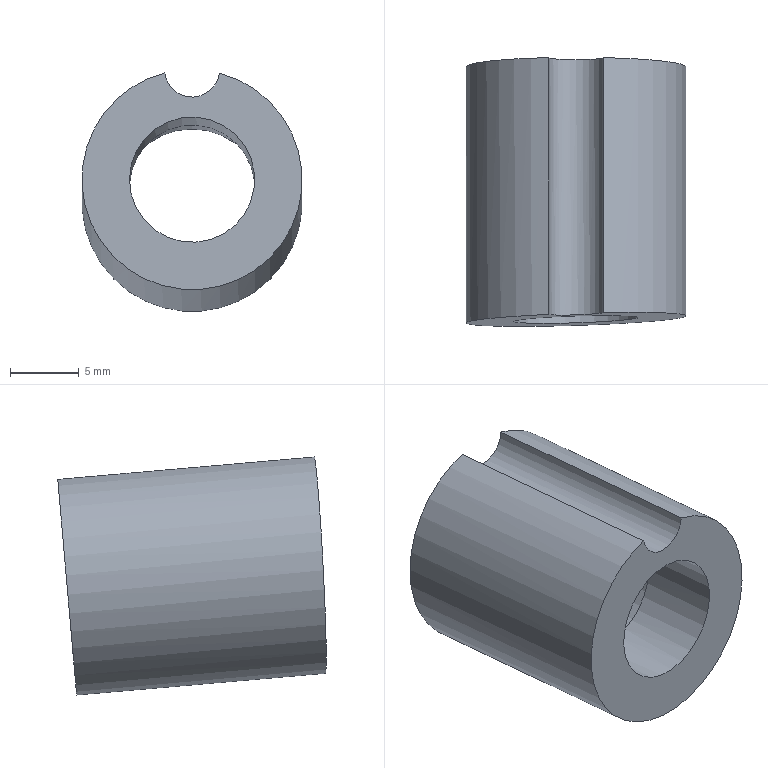Part | NX | features EKSD 16-20-7.100 2 | 1 solid | 7 faces | box 16 x 19.5 x 17.322 mm | volume 2113 mm3 | cylinder 4 | plane 3 | commonest cylinder face diameters 4 x1 9.1 x1 10.6 x1 16 x1
STEP:
#1=CARTESIAN_POINT('',(-563.09,-50.074,-37.699));
#2=VERTEX_POINT('',#1);
#3=CARTESIAN_POINT('',(-559.121,-50.074,-37.699));
#4=VERTEX_POINT('',#3);
#5=CARTESIAN_POINT('',(-561.105,-50.053,-37.45));
#6=DIRECTION('',(0.,-0.9962,0.08716));
#7=DIRECTION('',(0.,-0.08716,-0.9962));
#8=AXIS2_PLACEMENT_3D('',#5,#6,#7);
#9=CIRCLE('',#8,2.);
#10=EDGE_CURVE('',#2,#4,#9,.T.);
#11=ORIENTED_EDGE('',*,*,#10,.T.);
#12=CARTESIAN_POINT('',(-561.105,-50.75,-45.42));
#13=DIRECTION('',(0.,-0.9962,0.08716));
#14=DIRECTION('',(0.,-0.08716,-0.9962));
#15=AXIS2_PLACEMENT_3D('',#12,#13,#14);
#16=CIRCLE('',#15,8.);
#17=EDGE_CURVE('',#2,#4,#16,.T.);
#18=ORIENTED_EDGE('',*,*,#17,.F.);
#19=EDGE_LOOP('',(#11,#18));
#20=FACE_BOUND('',#19,.T.);
#21=CARTESIAN_POINT('',(-561.105,-50.288,-40.14));
#22=VERTEX_POINT('',#21);
#23=CARTESIAN_POINT('',(-561.105,-50.75,-45.42));
#24=DIRECTION('',(0.,0.9962,-0.08716));
#25=DIRECTION('',(0.,0.08716,0.9962));
#26=AXIS2_PLACEMENT_3D('',#23,#24,#25);
#27=CIRCLE('',#26,5.3);
#28=EDGE_CURVE('',#22,#22,#27,.T.);
#29=ORIENTED_EDGE('',*,*,#28,.F.);
#30=EDGE_LOOP('',(#29));
#31=FACE_BOUND('',#30,.T.);
#32=CARTESIAN_POINT('',(-561.105,-50.75,-45.42));
#33=DIRECTION('',(0.,0.9962,-0.08716));
#34=DIRECTION('',(0.,0.08716,0.9962));
#35=AXIS2_PLACEMENT_3D('',#32,#33,#34);
#36=PLANE('',#35);
#37=ADVANCED_FACE('',(#20,#31),#36,.T.);
#38=CARTESIAN_POINT('',(-559.121,-68.601,-36.078));
#39=VERTEX_POINT('',#38);
#40=CARTESIAN_POINT('',(-563.09,-68.729,-36.067));
#41=VERTEX_POINT('',#40);
#42=CARTESIAN_POINT('',(-561.105,-68.652,-35.823));
#43=DIRECTION('',(-0.03252,0.9981,-0.05307));
#44=DIRECTION('',(0.6892,-0.01607,-0.7244));
#45=AXIS2_PLACEMENT_3D('',#42,#43,#44);
#46=ELLIPSE('',#45,2.002,2.);
#47=EDGE_CURVE('',#39,#41,#46,.T.);
#48=ORIENTED_EDGE('',*,*,#47,.T.);
#49=CARTESIAN_POINT('',(-561.105,-69.077,-43.816));
#50=DIRECTION('',(-0.03252,0.9981,-0.05307));
#51=DIRECTION('',(0.6892,-0.01607,-0.7244));
#52=AXIS2_PLACEMENT_3D('',#49,#50,#51);
#53=ELLIPSE('',#52,8.009,8.);
#54=EDGE_CURVE('',#39,#41,#53,.T.);
#55=ORIENTED_EDGE('',*,*,#54,.F.);
#56=EDGE_LOOP('',(#48,#55));
#57=FACE_BOUND('',#56,.T.);
#58=CARTESIAN_POINT('',(-557.966,-69.15,-47.116));
#59=VERTEX_POINT('',#58);
#60=CARTESIAN_POINT('',(-561.105,-69.077,-43.816));
#61=DIRECTION('',(-0.03252,0.9981,-0.05307));
#62=DIRECTION('',(0.6892,-0.01607,-0.7244));
#63=AXIS2_PLACEMENT_3D('',#60,#61,#62);
#64=ELLIPSE('',#63,4.555,4.55);
#65=EDGE_CURVE('',#59,#59,#64,.F.);
#66=ORIENTED_EDGE('',*,*,#65,.F.);
#67=EDGE_LOOP('',(#66));
#68=FACE_BOUND('',#67,.T.);
#69=CARTESIAN_POINT('',(-422.194,-57.948,80.353));
#70=DIRECTION('',(-0.03252,0.9981,-0.05307));
#71=DIRECTION('',(0.05223,-0.05133,-0.9973));
#72=AXIS2_PLACEMENT_3D('',#69,#70,#71);
#73=PLANE('',#72);
#74=ADVANCED_FACE('',(#57,#68),#73,.F.);
#75=CARTESIAN_POINT('',(-559.121,-60.036,-36.828));
#76=DIRECTION('',(0.,0.9962,-0.08716));
#77=VECTOR('',#76,1000.);
#78=LINE('',#75,#77);
#79=EDGE_CURVE('',#39,#4,#78,.T.);
#80=ORIENTED_EDGE('',*,*,#79,.F.);
#81=ORIENTED_EDGE('',*,*,#54,.T.);
#82=CARTESIAN_POINT('',(-563.09,-60.036,-36.828));
#83=DIRECTION('',(0.,0.9962,-0.08716));
#84=VECTOR('',#83,1000.);
#85=LINE('',#82,#84);
#86=EDGE_CURVE('',#2,#41,#85,.F.);
#87=ORIENTED_EDGE('',*,*,#86,.F.);
#88=ORIENTED_EDGE('',*,*,#17,.T.);
#89=EDGE_LOOP('',(#80,#81,#87,#88));
#90=FACE_BOUND('',#89,.T.);
#91=CARTESIAN_POINT('',(-561.105,-70.674,-43.676));
#92=DIRECTION('',(0.,0.9962,-0.08716));
#93=DIRECTION('',(0.,0.08716,0.9962));
#94=AXIS2_PLACEMENT_3D('',#91,#92,#93);
#95=CYLINDRICAL_SURFACE('',#94,8.);
#96=ADVANCED_FACE('',(#90),#95,.T.);
#97=CARTESIAN_POINT('',(-561.105,-63.101,-48.906));
#98=VERTEX_POINT('',#97);
#99=CARTESIAN_POINT('',(-561.105,-62.704,-44.374));
#100=DIRECTION('',(0.,-0.9962,0.08716));
#101=DIRECTION('',(0.,-0.08716,-0.9962));
#102=AXIS2_PLACEMENT_3D('',#99,#100,#101);
#103=CIRCLE('',#102,4.55);
#104=EDGE_CURVE('',#98,#98,#103,.F.);
#105=ORIENTED_EDGE('',*,*,#104,.T.);
#106=EDGE_LOOP('',(#105));
#107=FACE_BOUND('',#106,.T.);
#108=ORIENTED_EDGE('',*,*,#65,.T.);
#109=EDGE_LOOP('',(#108));
#110=FACE_BOUND('',#109,.T.);
#111=CARTESIAN_POINT('',(-561.105,-71.67,-43.589));
#112=DIRECTION('',(0.,0.9962,-0.08716));
#113=DIRECTION('',(0.,0.08716,0.9962));
#114=AXIS2_PLACEMENT_3D('',#111,#112,#113);
#115=CYLINDRICAL_SURFACE('',#114,4.55);
#116=ADVANCED_FACE('',(#107,#110),#115,.F.);
#117=CARTESIAN_POINT('',(-561.105,-62.242,-39.094));
#118=VERTEX_POINT('',#117);
#119=CARTESIAN_POINT('',(-561.105,-62.704,-44.374));
#120=DIRECTION('',(0.,0.9962,-0.08716));
#121=DIRECTION('',(0.,0.08716,0.9962));
#122=AXIS2_PLACEMENT_3D('',#119,#120,#121);
#123=CIRCLE('',#122,5.3);
#124=EDGE_CURVE('',#118,#118,#123,.T.);
#125=ORIENTED_EDGE('',*,*,#124,.T.);
#126=EDGE_LOOP('',(#125));
#127=FACE_BOUND('',#126,.T.);
#128=ORIENTED_EDGE('',*,*,#104,.F.);
#129=EDGE_LOOP('',(#128));
#130=FACE_BOUND('',#129,.T.);
#131=CARTESIAN_POINT('',(-561.105,-62.704,-44.374));
#132=DIRECTION('',(0.,-0.9962,0.08716));
#133=DIRECTION('',(0.,-0.08716,-0.9962));
#134=AXIS2_PLACEMENT_3D('',#131,#132,#133);
#135=PLANE('',#134);
#136=ADVANCED_FACE('',(#127,#130),#135,.F.);
#137=ORIENTED_EDGE('',*,*,#28,.T.);
#138=EDGE_LOOP('',(#137));
#139=FACE_BOUND('',#138,.T.);
#140=ORIENTED_EDGE('',*,*,#124,.F.);
#141=EDGE_LOOP('',(#140));
#142=FACE_BOUND('',#141,.T.);
#143=CARTESIAN_POINT('',(-561.105,-62.704,-44.374));
#144=DIRECTION('',(0.,0.9962,-0.08716));
#145=DIRECTION('',(0.,0.08716,0.9962));
#146=AXIS2_PLACEMENT_3D('',#143,#144,#145);
#147=CYLINDRICAL_SURFACE('',#146,5.3);
#148=ADVANCED_FACE('',(#139,#142),#147,.F.);
#149=ORIENTED_EDGE('',*,*,#79,.T.);
#150=ORIENTED_EDGE('',*,*,#10,.F.);
#151=ORIENTED_EDGE('',*,*,#86,.T.);
#152=ORIENTED_EDGE('',*,*,#47,.F.);
#153=EDGE_LOOP('',(#149,#150,#151,#152));
#154=FACE_BOUND('',#153,.T.);
#155=CARTESIAN_POINT('',(-561.105,-69.977,-35.707));
#156=DIRECTION('',(0.,0.9962,-0.08716));
#157=DIRECTION('',(0.,0.08716,0.9962));
#158=AXIS2_PLACEMENT_3D('',#155,#156,#157);
#159=CYLINDRICAL_SURFACE('',#158,2.);
#160=ADVANCED_FACE('',(#154),#159,.F.);
#161=CLOSED_SHELL('',(#37,#74,#96,#116,#136,#148,#160));
#162=MANIFOLD_SOLID_BREP('',#161);
#163=(LENGTH_UNIT()NAMED_UNIT(*)SI_UNIT(.MILLI.,.METRE.));
#164=UNCERTAINTY_MEASURE_WITH_UNIT(LENGTH_MEASURE(0.00001),#163,'','');
#165=(NAMED_UNIT(*)PLANE_ANGLE_UNIT()SI_UNIT($,.RADIAN.));
#166=(NAMED_UNIT(*)SI_UNIT($,.STERADIAN.)SOLID_ANGLE_UNIT());
#167=(GEOMETRIC_REPRESENTATION_CONTEXT(3)GLOBAL_UNCERTAINTY_ASSIGNED_CONTEXT((#164))GLOBAL_UNIT_ASSIGNED_CONTEXT((#163,#165,#166))REPRESENTATION_CONTEXT('',''));
#168=ADVANCED_BREP_SHAPE_REPRESENTATION('',(#162),#167);